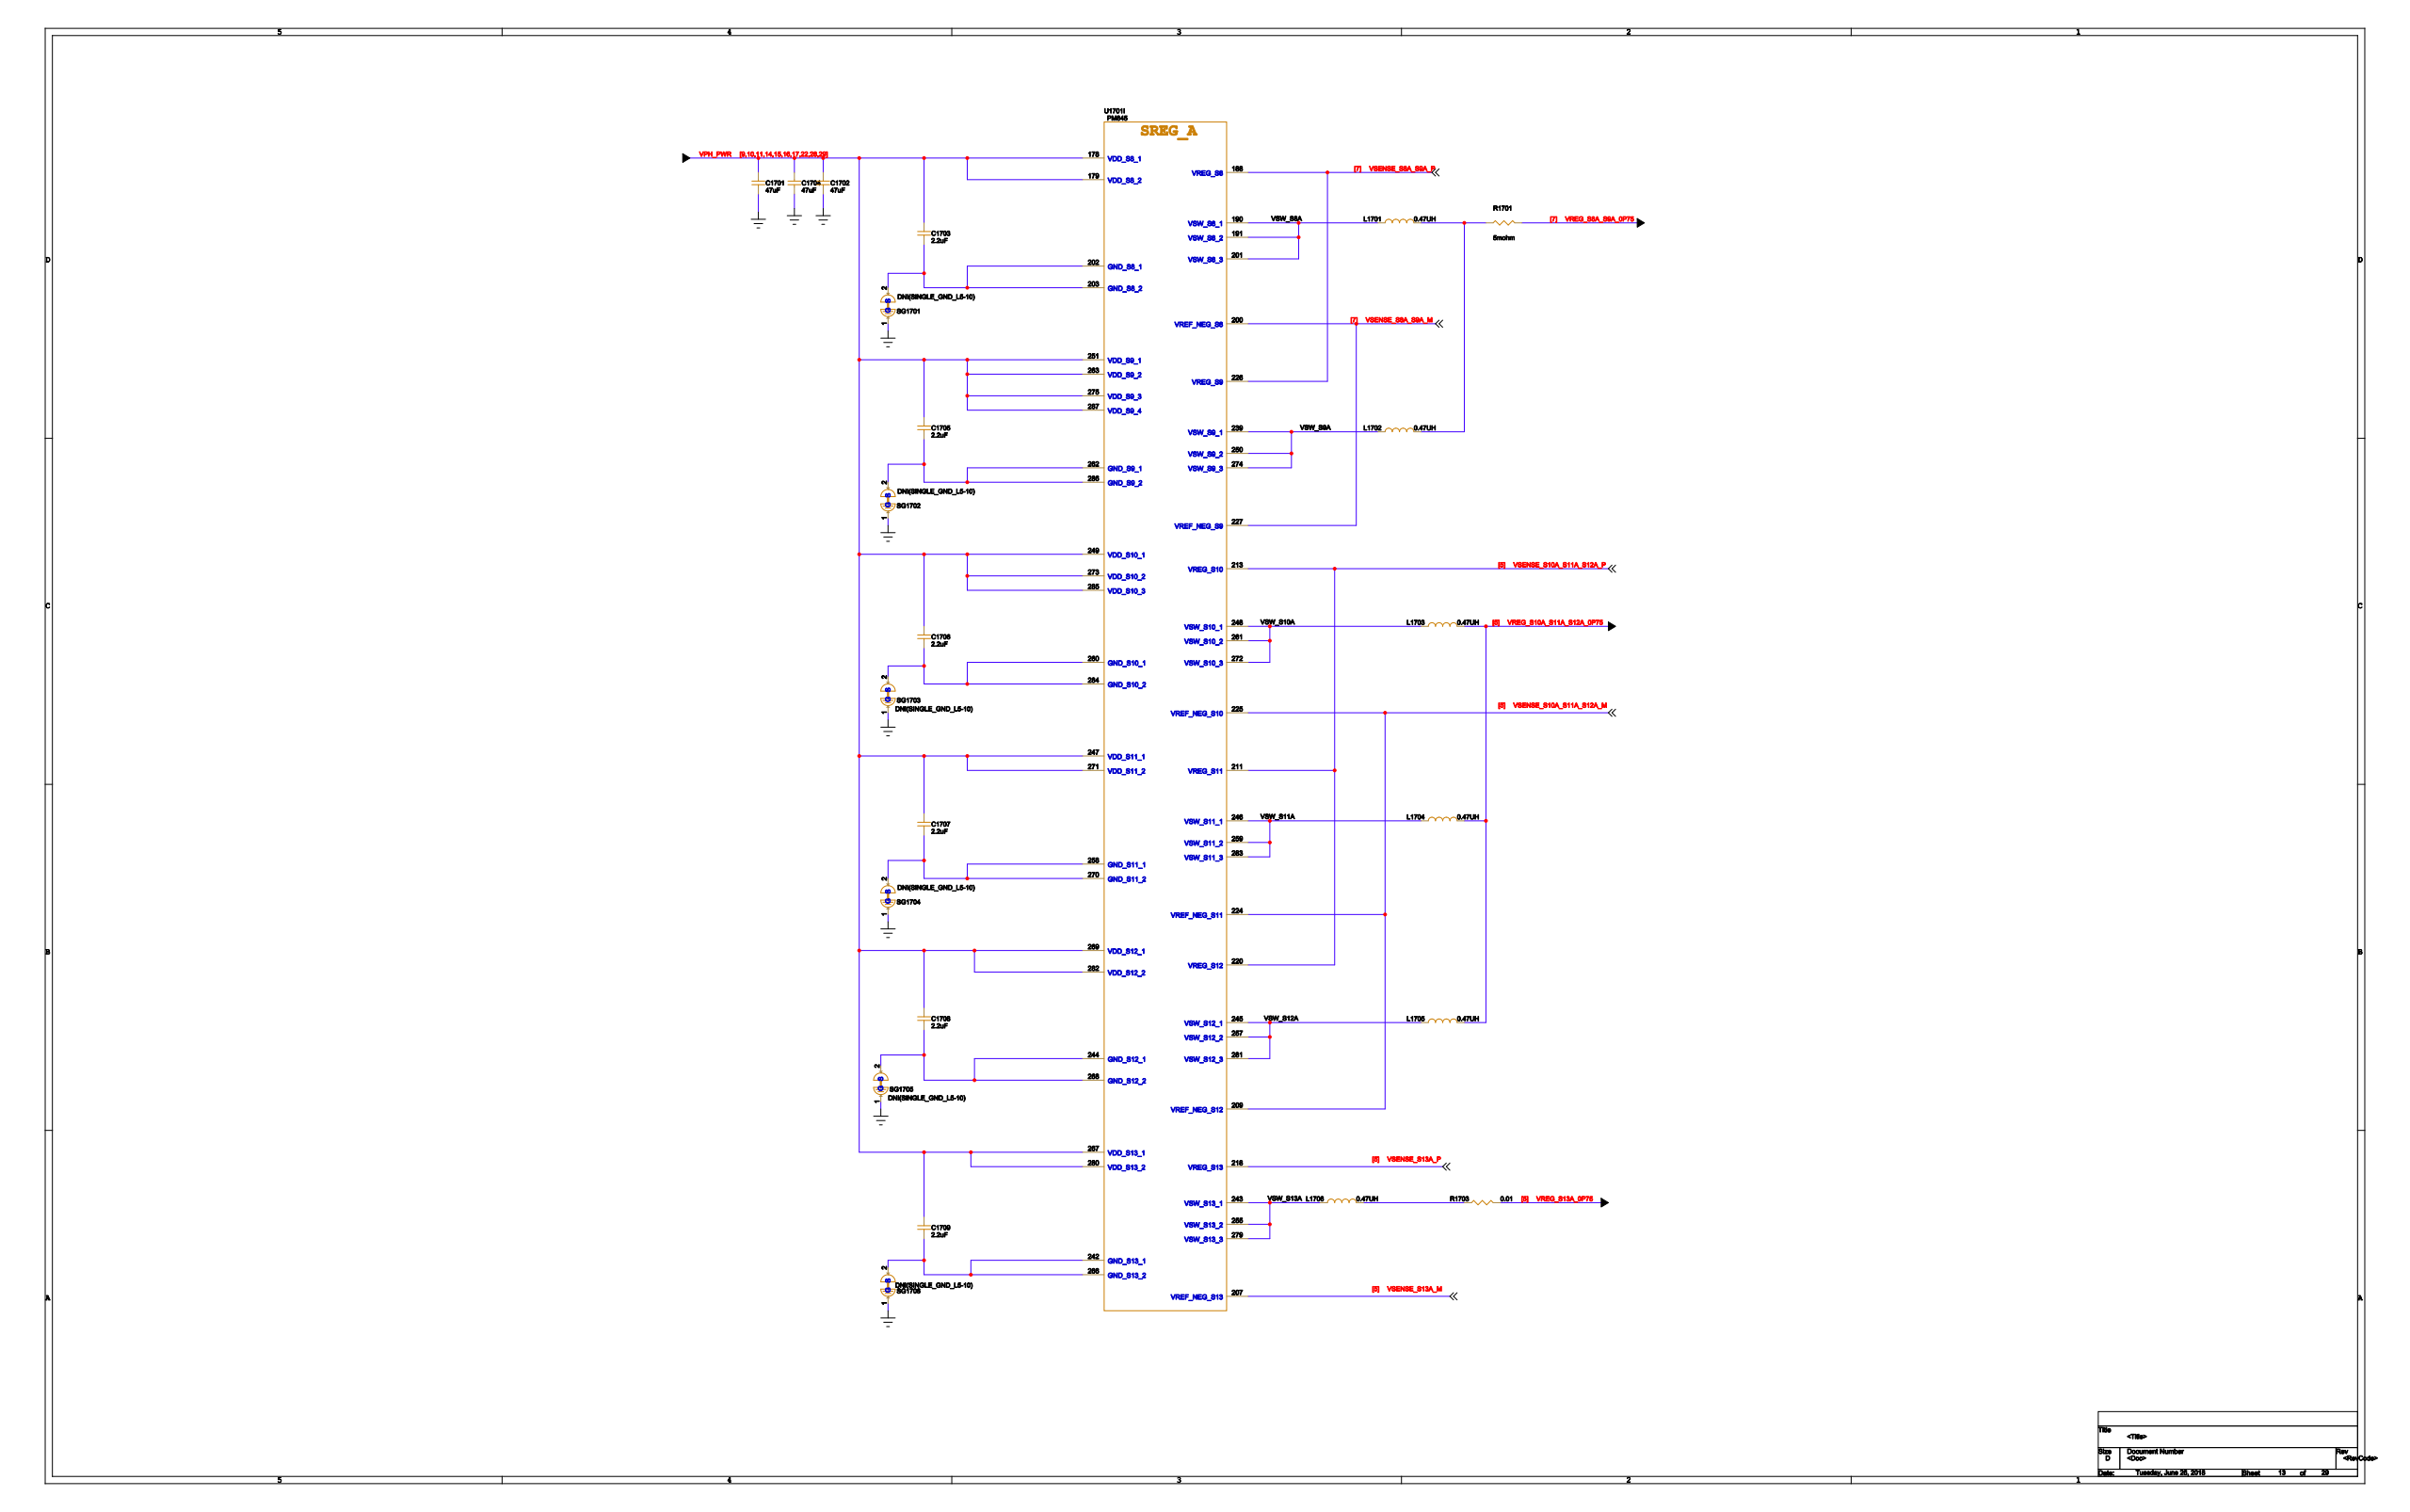Circuit board | Cadence Allegro | 802 parts | 566 nets | one sheet of the schematic
Parts on this sheet (reference | value | footprint):
C1701 | 47uF | C0805
C1702 | 47uF | C0805
C1703 | 2.2uF | 0402-BIG
C1704 | 47uF | C0805
C1705 | 2.2uF | 0402-BIG
C1706 | 2.2uF | 0402-BIG
C1707 | 2.2uF | 0402-BIG
C1708 | 2.2uF | 0402-BIG
C1709 | 2.2uF | 0402-BIG
L1701 | 0.47UH | L2016_MEKK2016
L1702 | 0.47UH | L2016_MEKK2016
L1703 | 0.47UH | L2016_MEKK2016
L1704 | 0.47UH | L2016_MEKK2016
L1705 | 0.47UH | L2016_MEKK2016
L1706 | 0.47UH | L2016_MEKK2016
R1701 | 5mohm | R0805_PE0805FRE470R005Z
R1703 | 0.01 | R0603
SG1701 | DNI(SINGLE_GND_L5-10) | GND_L5-10
SG1702 | DNI(SINGLE_GND_L5-10) | GND_L5-10
SG1703 | DNI(SINGLE_GND_L5-10) | GND_L5-10
SG1704 | DNI(SINGLE_GND_L5-10) | GND_L5-10
SG1705 | DNI(SINGLE_GND_L5-10) | GND_L5-10
SG1706 | DNI(SINGLE_GND_L5-10) | GND_L5-10
U1701 | PM845 | PM8998
Nets of these parts (net: part-pin ...):
GND: C1701-2 C1702-2 C1704-2 SG1701-1 SG1702-1 SG1703-1 SG1704-1 SG1705-1 SG1706-1
VPH_PWR: C1701-1 C1702-1 C1703-1 C1704-1 C1705-1 C1706-1 C1707-1 C1708-1 C1709-1 U1701-178 U1701-179 U1701-247 U1701-249 U1701-251 U1701-263 U1701-267 U1701-269 U1701-271 U1701-273 U1701-275 U1701-280 U1701-282 U1701-285 U1701-287
N189374: L1706-2 R1703-1
VREG_S13A_0P75: R1703-2
VREG_S10A_S11A_S12A_0P75: L1703-2 L1704-2 L1705-2
VREG_S8A_S9A_0P75: R1701-2
N189574: C1703-2 SG1701-2 U1701-202 U1701-203
N189622: C1705-2 SG1702-2 U1701-262 U1701-286
N189702: C1706-2 SG1703-2 U1701-260 U1701-284
N189758: C1707-2 SG1704-2 U1701-258 U1701-270
N189816: C1708-2 SG1705-2 U1701-244 U1701-268
N189836: C1709-2 SG1706-2 U1701-242 U1701-266
VSW_S8A: L1701-1 U1701-190 U1701-191 U1701-201
N189510: L1701-2 L1702-2 R1701-1
VSW_S9A: L1702-1 U1701-239 U1701-250 U1701-274
VSW_S10A: L1703-1 U1701-248 U1701-261 U1701-272
VSW_S11A: L1704-1 U1701-246 U1701-259 U1701-283
VSW_S12A: L1705-1 U1701-245 U1701-257 U1701-281
VSW_S13A: L1706-1 U1701-243 U1701-255 U1701-279
VSENSE_S10A_S11A_S12A_M: U1701-209 U1701-224 U1701-225
VSENSE_S10A_S11A_S12A_P: U1701-211 U1701-213 U1701-220
VSENSE_S13A_M: U1701-207
VSENSE_S13A_P: U1701-218
VSENSE_S8A_S9A_M: U1701-200 U1701-227
VSENSE_S8A_S9A_P: U1701-188 U1701-226